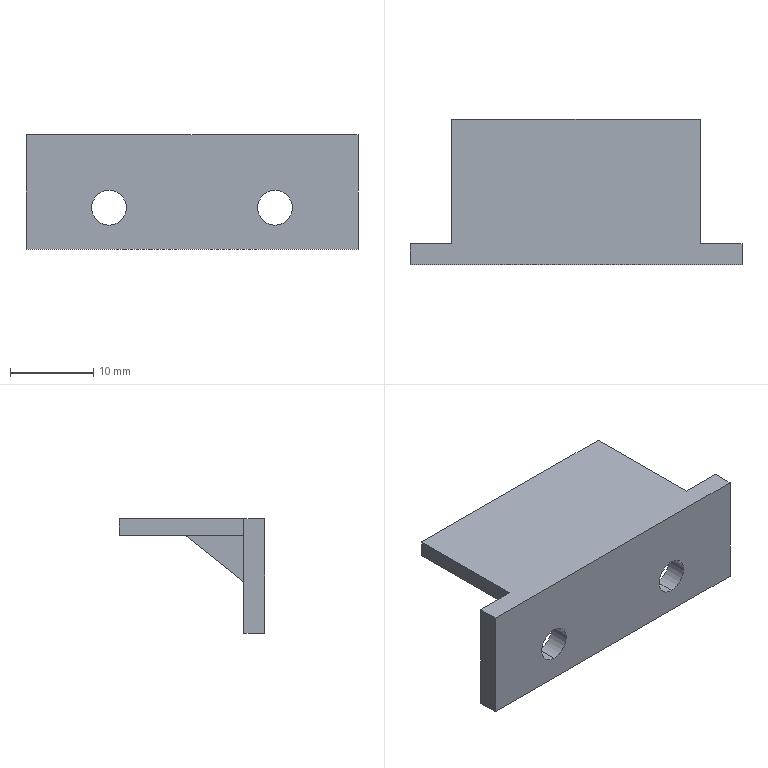Part | SolidWorks | features BaseBody 1 | 1 solid | 17 faces | box 40 x 17.5 x 13.8 mm | volume 2505 mm3 | plane 13 | cylinder 4 | commonest cylinder face diameters 4.2 x4
STEP:
#1=CARTESIAN_POINT('',(269.946,-4030.973,2013.371));
#2=VERTEX_POINT('',#1);
#3=CARTESIAN_POINT('',(269.946,-4030.973,2017.571));
#4=VERTEX_POINT('',#3);
#5=CARTESIAN_POINT('',(269.946,-4030.973,2015.471));
#6=DIRECTION('',(0.,1.,0.));
#7=DIRECTION('',(0.,0.,1.));
#8=AXIS2_PLACEMENT_3D('',#5,#6,#7);
#9=CIRCLE('',#8,2.1);
#10=EDGE_CURVE('',#2,#4,#9,.T.);
#11=ORIENTED_EDGE('',*,*,#10,.F.);
#12=CARTESIAN_POINT('',(269.946,-4028.473,2013.371));
#13=VERTEX_POINT('',#12);
#14=CARTESIAN_POINT('',(269.946,-4034.473,2013.371));
#15=DIRECTION('',(0.,1.,0.));
#16=VECTOR('',#15,1000.);
#17=LINE('',#14,#16);
#18=EDGE_CURVE('',#2,#13,#17,.T.);
#19=ORIENTED_EDGE('',*,*,#18,.T.);
#20=CARTESIAN_POINT('',(269.946,-4028.473,2017.571));
#21=VERTEX_POINT('',#20);
#22=CARTESIAN_POINT('',(269.946,-4028.473,2015.471));
#23=DIRECTION('',(0.,1.,0.));
#24=DIRECTION('',(0.,0.,1.));
#25=AXIS2_PLACEMENT_3D('',#22,#23,#24);
#26=CIRCLE('',#25,2.1);
#27=EDGE_CURVE('',#13,#21,#26,.T.);
#28=ORIENTED_EDGE('',*,*,#27,.T.);
#29=CARTESIAN_POINT('',(269.946,-4034.473,2017.571));
#30=DIRECTION('',(0.,1.,0.));
#31=VECTOR('',#30,1000.);
#32=LINE('',#29,#31);
#33=EDGE_CURVE('',#4,#21,#32,.T.);
#34=ORIENTED_EDGE('',*,*,#33,.F.);
#35=EDGE_LOOP('',(#11,#19,#28,#34));
#36=FACE_OUTER_BOUND('',#35,.T.);
#37=CARTESIAN_POINT('',(269.946,-4034.473,2015.471));
#38=DIRECTION('',(0.,1.,0.));
#39=DIRECTION('',(0.,0.,1.));
#40=AXIS2_PLACEMENT_3D('',#37,#38,#39);
#41=CYLINDRICAL_SURFACE('',#40,2.1);
#42=ADVANCED_FACE('',(#36),#41,.F.);
#43=CARTESIAN_POINT('',(249.946,-4030.973,2013.371));
#44=VERTEX_POINT('',#43);
#45=CARTESIAN_POINT('',(249.946,-4030.973,2017.571));
#46=VERTEX_POINT('',#45);
#47=CARTESIAN_POINT('',(249.946,-4030.973,2015.471));
#48=DIRECTION('',(0.,1.,0.));
#49=DIRECTION('',(0.,0.,1.));
#50=AXIS2_PLACEMENT_3D('',#47,#48,#49);
#51=CIRCLE('',#50,2.1);
#52=EDGE_CURVE('',#44,#46,#51,.T.);
#53=ORIENTED_EDGE('',*,*,#52,.F.);
#54=CARTESIAN_POINT('',(249.946,-4028.473,2013.371));
#55=VERTEX_POINT('',#54);
#56=CARTESIAN_POINT('',(249.946,-4034.473,2013.371));
#57=DIRECTION('',(0.,1.,0.));
#58=VECTOR('',#57,1000.);
#59=LINE('',#56,#58);
#60=EDGE_CURVE('',#44,#55,#59,.T.);
#61=ORIENTED_EDGE('',*,*,#60,.T.);
#62=CARTESIAN_POINT('',(249.946,-4028.473,2017.571));
#63=VERTEX_POINT('',#62);
#64=CARTESIAN_POINT('',(249.946,-4028.473,2015.471));
#65=DIRECTION('',(0.,1.,0.));
#66=DIRECTION('',(0.,0.,1.));
#67=AXIS2_PLACEMENT_3D('',#64,#65,#66);
#68=CIRCLE('',#67,2.1);
#69=EDGE_CURVE('',#55,#63,#68,.T.);
#70=ORIENTED_EDGE('',*,*,#69,.T.);
#71=CARTESIAN_POINT('',(249.946,-4034.473,2017.571));
#72=DIRECTION('',(0.,1.,0.));
#73=VECTOR('',#72,1000.);
#74=LINE('',#71,#73);
#75=EDGE_CURVE('',#46,#63,#74,.T.);
#76=ORIENTED_EDGE('',*,*,#75,.F.);
#77=EDGE_LOOP('',(#53,#61,#70,#76));
#78=FACE_OUTER_BOUND('',#77,.T.);
#79=CARTESIAN_POINT('',(249.946,-4034.473,2015.471));
#80=DIRECTION('',(0.,1.,0.));
#81=DIRECTION('',(0.,0.,1.));
#82=AXIS2_PLACEMENT_3D('',#79,#80,#81);
#83=CYLINDRICAL_SURFACE('',#82,2.1);
#84=ADVANCED_FACE('',(#78),#83,.F.);
#85=CARTESIAN_POINT('',(244.946,-4028.473,2024.271));
#86=VERTEX_POINT('',#85);
#87=CARTESIAN_POINT('',(239.946,-4028.473,2024.271));
#88=VERTEX_POINT('',#87);
#89=CARTESIAN_POINT('',(259.946,-4028.473,2024.271));
#90=DIRECTION('',(-1.,0.,0.));
#91=VECTOR('',#90,1000.);
#92=LINE('',#89,#91);
#93=EDGE_CURVE('',#86,#88,#92,.T.);
#94=ORIENTED_EDGE('',*,*,#93,.T.);
#95=CARTESIAN_POINT('',(239.946,-4030.973,2024.271));
#96=VERTEX_POINT('',#95);
#97=CARTESIAN_POINT('',(239.946,-4028.473,2024.271));
#98=DIRECTION('',(0.,-1.,0.));
#99=VECTOR('',#98,1000.);
#100=LINE('',#97,#99);
#101=EDGE_CURVE('',#88,#96,#100,.T.);
#102=ORIENTED_EDGE('',*,*,#101,.T.);
#103=CARTESIAN_POINT('',(279.946,-4030.973,2024.271));
#104=VERTEX_POINT('',#103);
#105=CARTESIAN_POINT('',(259.946,-4030.973,2024.271));
#106=DIRECTION('',(1.,0.,0.));
#107=VECTOR('',#106,1000.);
#108=LINE('',#105,#107);
#109=EDGE_CURVE('',#96,#104,#108,.T.);
#110=ORIENTED_EDGE('',*,*,#109,.T.);
#111=CARTESIAN_POINT('',(279.946,-4028.473,2024.271));
#112=VERTEX_POINT('',#111);
#113=CARTESIAN_POINT('',(279.946,-4028.473,2024.271));
#114=DIRECTION('',(0.,1.,0.));
#115=VECTOR('',#114,1000.);
#116=LINE('',#113,#115);
#117=EDGE_CURVE('',#104,#112,#116,.T.);
#118=ORIENTED_EDGE('',*,*,#117,.T.);
#119=CARTESIAN_POINT('',(274.946,-4028.473,2024.271));
#120=VERTEX_POINT('',#119);
#121=CARTESIAN_POINT('',(259.946,-4028.473,2024.271));
#122=DIRECTION('',(-1.,0.,0.));
#123=VECTOR('',#122,1000.);
#124=LINE('',#121,#123);
#125=EDGE_CURVE('',#112,#120,#124,.T.);
#126=ORIENTED_EDGE('',*,*,#125,.T.);
#127=CARTESIAN_POINT('',(274.946,-4013.473,2024.271));
#128=VERTEX_POINT('',#127);
#129=CARTESIAN_POINT('',(274.946,-4028.473,2024.271));
#130=DIRECTION('',(0.,1.,0.));
#131=VECTOR('',#130,1000.);
#132=LINE('',#129,#131);
#133=EDGE_CURVE('',#120,#128,#132,.T.);
#134=ORIENTED_EDGE('',*,*,#133,.T.);
#135=CARTESIAN_POINT('',(244.946,-4013.473,2024.271));
#136=VERTEX_POINT('',#135);
#137=CARTESIAN_POINT('',(259.946,-4013.473,2024.271));
#138=DIRECTION('',(-1.,0.,0.));
#139=VECTOR('',#138,1000.);
#140=LINE('',#137,#139);
#141=EDGE_CURVE('',#128,#136,#140,.T.);
#142=ORIENTED_EDGE('',*,*,#141,.T.);
#143=CARTESIAN_POINT('',(244.946,-4028.473,2024.271));
#144=DIRECTION('',(0.,-1.,0.));
#145=VECTOR('',#144,1000.);
#146=LINE('',#143,#145);
#147=EDGE_CURVE('',#136,#86,#146,.T.);
#148=ORIENTED_EDGE('',*,*,#147,.T.);
#149=EDGE_LOOP('',(#94,#102,#110,#118,#126,#134,#142,#148));
#150=FACE_OUTER_BOUND('',#149,.T.);
#151=CARTESIAN_POINT('',(259.946,-4028.473,2024.271));
#152=DIRECTION('',(0.,0.,1.));
#153=DIRECTION('',(0.,-1.,0.));
#154=AXIS2_PLACEMENT_3D('',#151,#152,#153);
#155=PLANE('',#154);
#156=ADVANCED_FACE('',(#150),#155,.T.);
#157=CARTESIAN_POINT('',(239.946,-4030.973,2010.471));
#158=VERTEX_POINT('',#157);
#159=CARTESIAN_POINT('',(239.946,-4030.973,2024.271));
#160=DIRECTION('',(0.,0.,1.));
#161=VECTOR('',#160,1000.);
#162=LINE('',#159,#161);
#163=EDGE_CURVE('',#158,#96,#162,.T.);
#164=ORIENTED_EDGE('',*,*,#163,.T.);
#165=ORIENTED_EDGE('',*,*,#101,.F.);
#166=CARTESIAN_POINT('',(239.946,-4028.473,2010.471));
#167=VERTEX_POINT('',#166);
#168=CARTESIAN_POINT('',(239.946,-4028.473,2024.271));
#169=DIRECTION('',(0.,0.,-1.));
#170=VECTOR('',#169,1000.);
#171=LINE('',#168,#170);
#172=EDGE_CURVE('',#88,#167,#171,.T.);
#173=ORIENTED_EDGE('',*,*,#172,.T.);
#174=CARTESIAN_POINT('',(239.946,-4034.473,2010.471));
#175=DIRECTION('',(0.,-1.,0.));
#176=VECTOR('',#175,1000.);
#177=LINE('',#174,#176);
#178=EDGE_CURVE('',#167,#158,#177,.T.);
#179=ORIENTED_EDGE('',*,*,#178,.T.);
#180=EDGE_LOOP('',(#164,#165,#173,#179));
#181=FACE_OUTER_BOUND('',#180,.T.);
#182=CARTESIAN_POINT('',(239.946,-4034.473,2024.271));
#183=DIRECTION('',(-1.,0.,0.));
#184=DIRECTION('',(0.,-1.,0.));
#185=AXIS2_PLACEMENT_3D('',#182,#183,#184);
#186=PLANE('',#185);
#187=ADVANCED_FACE('',(#181),#186,.T.);
#188=CARTESIAN_POINT('',(267.446,-4028.473,2016.671));
#189=VERTEX_POINT('',#188);
#190=CARTESIAN_POINT('',(252.446,-4028.473,2016.671));
#191=VERTEX_POINT('',#190);
#192=CARTESIAN_POINT('',(279.946,-4028.473,2016.671));
#193=DIRECTION('',(-1.,0.,0.));
#194=VECTOR('',#193,1000.);
#195=LINE('',#192,#194);
#196=EDGE_CURVE('',#189,#191,#195,.T.);
#197=ORIENTED_EDGE('',*,*,#196,.F.);
#198=CARTESIAN_POINT('',(267.446,-4028.473,2022.271));
#199=VERTEX_POINT('',#198);
#200=CARTESIAN_POINT('',(267.446,-4028.473,2024.271));
#201=DIRECTION('',(0.,0.,-1.));
#202=VECTOR('',#201,1000.);
#203=LINE('',#200,#202);
#204=EDGE_CURVE('',#199,#189,#203,.T.);
#205=ORIENTED_EDGE('',*,*,#204,.F.);
#206=CARTESIAN_POINT('',(274.946,-4028.473,2022.271));
#207=VERTEX_POINT('',#206);
#208=CARTESIAN_POINT('',(279.946,-4028.473,2022.271));
#209=DIRECTION('',(-1.,0.,0.));
#210=VECTOR('',#209,1000.);
#211=LINE('',#208,#210);
#212=EDGE_CURVE('',#207,#199,#211,.T.);
#213=ORIENTED_EDGE('',*,*,#212,.F.);
#214=CARTESIAN_POINT('',(274.946,-4028.473,2024.271));
#215=DIRECTION('',(0.,0.,-1.));
#216=VECTOR('',#215,1000.);
#217=LINE('',#214,#216);
#218=EDGE_CURVE('',#120,#207,#217,.T.);
#219=ORIENTED_EDGE('',*,*,#218,.F.);
#220=ORIENTED_EDGE('',*,*,#125,.F.);
#221=CARTESIAN_POINT('',(279.946,-4028.473,2010.471));
#222=VERTEX_POINT('',#221);
#223=CARTESIAN_POINT('',(279.946,-4028.473,2024.271));
#224=DIRECTION('',(0.,0.,1.));
#225=VECTOR('',#224,1000.);
#226=LINE('',#223,#225);
#227=EDGE_CURVE('',#222,#112,#226,.T.);
#228=ORIENTED_EDGE('',*,*,#227,.F.);
#229=CARTESIAN_POINT('',(279.946,-4028.473,2010.471));
#230=DIRECTION('',(1.,0.,0.));
#231=VECTOR('',#230,1000.);
#232=LINE('',#229,#231);
#233=EDGE_CURVE('',#167,#222,#232,.T.);
#234=ORIENTED_EDGE('',*,*,#233,.F.);
#235=ORIENTED_EDGE('',*,*,#172,.F.);
#236=ORIENTED_EDGE('',*,*,#93,.F.);
#237=CARTESIAN_POINT('',(244.946,-4028.473,2022.271));
#238=VERTEX_POINT('',#237);
#239=CARTESIAN_POINT('',(244.946,-4028.473,2024.271));
#240=DIRECTION('',(0.,0.,1.));
#241=VECTOR('',#240,1000.);
#242=LINE('',#239,#241);
#243=EDGE_CURVE('',#238,#86,#242,.T.);
#244=ORIENTED_EDGE('',*,*,#243,.F.);
#245=CARTESIAN_POINT('',(252.446,-4028.473,2022.271));
#246=VERTEX_POINT('',#245);
#247=CARTESIAN_POINT('',(279.946,-4028.473,2022.271));
#248=DIRECTION('',(-1.,0.,0.));
#249=VECTOR('',#248,1000.);
#250=LINE('',#247,#249);
#251=EDGE_CURVE('',#246,#238,#250,.T.);
#252=ORIENTED_EDGE('',*,*,#251,.F.);
#253=CARTESIAN_POINT('',(252.446,-4028.473,2024.271));
#254=DIRECTION('',(0.,0.,1.));
#255=VECTOR('',#254,1000.);
#256=LINE('',#253,#255);
#257=EDGE_CURVE('',#191,#246,#256,.T.);
#258=ORIENTED_EDGE('',*,*,#257,.F.);
#259=EDGE_LOOP('',(#197,#205,#213,#219,#220,#228,#234,#235,#236,#244,#252,#258));
#260=FACE_OUTER_BOUND('',#259,.T.);
#261=CARTESIAN_POINT('',(269.946,-4028.473,2015.471));
#262=DIRECTION('',(0.,1.,0.));
#263=DIRECTION('',(0.,0.,1.));
#264=AXIS2_PLACEMENT_3D('',#261,#262,#263);
#265=CIRCLE('',#264,2.1);
#266=EDGE_CURVE('',#21,#13,#265,.T.);
#267=ORIENTED_EDGE('',*,*,#266,.F.);
#268=ORIENTED_EDGE('',*,*,#27,.F.);
#269=EDGE_LOOP('',(#267,#268));
#270=FACE_BOUND('',#269,.T.);
#271=CARTESIAN_POINT('',(249.946,-4028.473,2015.471));
#272=DIRECTION('',(0.,1.,0.));
#273=DIRECTION('',(0.,0.,1.));
#274=AXIS2_PLACEMENT_3D('',#271,#272,#273);
#275=CIRCLE('',#274,2.1);
#276=EDGE_CURVE('',#63,#55,#275,.T.);
#277=ORIENTED_EDGE('',*,*,#276,.F.);
#278=ORIENTED_EDGE('',*,*,#69,.F.);
#279=EDGE_LOOP('',(#277,#278));
#280=FACE_BOUND('',#279,.T.);
#281=CARTESIAN_POINT('',(279.946,-4028.473,2024.271));
#282=DIRECTION('',(0.,-1.,0.));
#283=DIRECTION('',(0.,0.,-1.));
#284=AXIS2_PLACEMENT_3D('',#281,#282,#283);
#285=PLANE('',#284);
#286=ADVANCED_FACE('',(#260,#270,#280),#285,.F.);
#287=CARTESIAN_POINT('',(244.946,-4013.473,2022.271));
#288=VERTEX_POINT('',#287);
#289=CARTESIAN_POINT('',(244.946,-4013.473,2024.271));
#290=DIRECTION('',(0.,0.,-1.));
#291=VECTOR('',#290,1000.);
#292=LINE('',#289,#291);
#293=EDGE_CURVE('',#136,#288,#292,.T.);
#294=ORIENTED_EDGE('',*,*,#293,.T.);
#295=CARTESIAN_POINT('',(244.946,-4013.473,2022.271));
#296=DIRECTION('',(0.,-1.,0.));
#297=VECTOR('',#296,1000.);
#298=LINE('',#295,#297);
#299=EDGE_CURVE('',#288,#238,#298,.T.);
#300=ORIENTED_EDGE('',*,*,#299,.T.);
#301=ORIENTED_EDGE('',*,*,#243,.T.);
#302=ORIENTED_EDGE('',*,*,#147,.F.);
#303=EDGE_LOOP('',(#294,#300,#301,#302));
#304=FACE_OUTER_BOUND('',#303,.T.);
#305=CARTESIAN_POINT('',(244.946,-4013.473,2024.271));
#306=DIRECTION('',(-1.,0.,0.));
#307=DIRECTION('',(0.,-1.,0.));
#308=AXIS2_PLACEMENT_3D('',#305,#306,#307);
#309=PLANE('',#308);
#310=ADVANCED_FACE('',(#304),#309,.T.);
#311=ORIENTED_EDGE('',*,*,#141,.F.);
#312=CARTESIAN_POINT('',(274.946,-4013.473,2022.271));
#313=VERTEX_POINT('',#312);
#314=CARTESIAN_POINT('',(274.946,-4013.473,2024.271));
#315=DIRECTION('',(0.,0.,-1.));
#316=VECTOR('',#315,1000.);
#317=LINE('',#314,#316);
#318=EDGE_CURVE('',#128,#313,#317,.T.);
#319=ORIENTED_EDGE('',*,*,#318,.T.);
#320=CARTESIAN_POINT('',(274.946,-4013.473,2022.271));
#321=DIRECTION('',(-1.,0.,0.));
#322=VECTOR('',#321,1000.);
#323=LINE('',#320,#322);
#324=EDGE_CURVE('',#313,#288,#323,.T.);
#325=ORIENTED_EDGE('',*,*,#324,.T.);
#326=ORIENTED_EDGE('',*,*,#293,.F.);
#327=EDGE_LOOP('',(#311,#319,#325,#326));
#328=FACE_OUTER_BOUND('',#327,.T.);
#329=CARTESIAN_POINT('',(274.946,-4013.473,2024.271));
#330=DIRECTION('',(0.,1.,0.));
#331=DIRECTION('',(0.,0.,1.));
#332=AXIS2_PLACEMENT_3D('',#329,#330,#331);
#333=PLANE('',#332);
#334=ADVANCED_FACE('',(#328),#333,.T.);
#335=ORIENTED_EDGE('',*,*,#318,.F.);
#336=ORIENTED_EDGE('',*,*,#133,.F.);
#337=ORIENTED_EDGE('',*,*,#218,.T.);
#338=CARTESIAN_POINT('',(274.946,-4043.473,2022.271));
#339=DIRECTION('',(0.,1.,0.));
#340=VECTOR('',#339,1000.);
#341=LINE('',#338,#340);
#342=EDGE_CURVE('',#207,#313,#341,.T.);
#343=ORIENTED_EDGE('',*,*,#342,.T.);
#344=EDGE_LOOP('',(#335,#336,#337,#343));
#345=FACE_OUTER_BOUND('',#344,.T.);
#346=CARTESIAN_POINT('',(274.946,-4043.473,2024.271));
#347=DIRECTION('',(1.,0.,0.));
#348=DIRECTION('',(0.,1.,0.));
#349=AXIS2_PLACEMENT_3D('',#346,#347,#348);
#350=PLANE('',#349);
#351=ADVANCED_FACE('',(#345),#350,.T.);
#352=CARTESIAN_POINT('',(279.946,-4030.973,2010.471));
#353=VERTEX_POINT('',#352);
#354=CARTESIAN_POINT('',(279.946,-4030.973,2006.271));
#355=DIRECTION('',(0.,0.,-1.));
#356=VECTOR('',#355,1000.);
#357=LINE('',#354,#356);
#358=EDGE_CURVE('',#104,#353,#357,.T.);
#359=ORIENTED_EDGE('',*,*,#358,.T.);
#360=CARTESIAN_POINT('',(279.946,-4034.473,2010.471));
#361=DIRECTION('',(0.,1.,0.));
#362=VECTOR('',#361,1000.);
#363=LINE('',#360,#362);
#364=EDGE_CURVE('',#353,#222,#363,.T.);
#365=ORIENTED_EDGE('',*,*,#364,.T.);
#366=ORIENTED_EDGE('',*,*,#227,.T.);
#367=ORIENTED_EDGE('',*,*,#117,.F.);
#368=EDGE_LOOP('',(#359,#365,#366,#367));
#369=FACE_OUTER_BOUND('',#368,.T.);
#370=CARTESIAN_POINT('',(279.946,-4034.473,2006.271));
#371=DIRECTION('',(1.,0.,0.));
#372=DIRECTION('',(0.,1.,0.));
#373=AXIS2_PLACEMENT_3D('',#370,#371,#372);
#374=PLANE('',#373);
#375=ADVANCED_FACE('',(#369),#374,.T.);
#376=CARTESIAN_POINT('',(269.946,-4030.973,2015.471));
#377=DIRECTION('',(0.,1.,0.));
#378=DIRECTION('',(0.,0.,1.));
#379=AXIS2_PLACEMENT_3D('',#376,#377,#378);
#380=CIRCLE('',#379,2.1);
#381=EDGE_CURVE('',#4,#2,#380,.T.);
#382=ORIENTED_EDGE('',*,*,#381,.T.);
#383=ORIENTED_EDGE('',*,*,#10,.T.);
#384=EDGE_LOOP('',(#382,#383));
#385=FACE_BOUND('',#384,.T.);
#386=CARTESIAN_POINT('',(249.946,-4030.973,2015.471));
#387=DIRECTION('',(0.,1.,0.));
#388=DIRECTION('',(0.,0.,1.));
#389=AXIS2_PLACEMENT_3D('',#386,#387,#388);
#390=CIRCLE('',#389,2.1);
#391=EDGE_CURVE('',#46,#44,#390,.T.);
#392=ORIENTED_EDGE('',*,*,#391,.T.);
#393=ORIENTED_EDGE('',*,*,#52,.T.);
#394=EDGE_LOOP('',(#392,#393));
#395=FACE_BOUND('',#394,.T.);
#396=ORIENTED_EDGE('',*,*,#109,.F.);
#397=ORIENTED_EDGE('',*,*,#163,.F.);
#398=CARTESIAN_POINT('',(259.946,-4030.973,2010.471));
#399=DIRECTION('',(1.,0.,0.));
#400=VECTOR('',#399,1000.);
#401=LINE('',#398,#400);
#402=EDGE_CURVE('',#158,#353,#401,.T.);
#403=ORIENTED_EDGE('',*,*,#402,.T.);
#404=ORIENTED_EDGE('',*,*,#358,.F.);
#405=EDGE_LOOP('',(#396,#397,#403,#404));
#406=FACE_OUTER_BOUND('',#405,.T.);
#407=CARTESIAN_POINT('',(259.946,-4030.973,2015.271));
#408=DIRECTION('',(0.,-1.,0.));
#409=DIRECTION('',(0.,0.,-1.));
#410=AXIS2_PLACEMENT_3D('',#407,#408,#409);
#411=PLANE('',#410);
#412=ADVANCED_FACE('',(#385,#395,#406),#411,.T.);
#413=ORIENTED_EDGE('',*,*,#402,.F.);
#414=ORIENTED_EDGE('',*,*,#178,.F.);
#415=ORIENTED_EDGE('',*,*,#233,.T.);
#416=ORIENTED_EDGE('',*,*,#364,.F.);
#417=EDGE_LOOP('',(#413,#414,#415,#416));
#418=FACE_OUTER_BOUND('',#417,.T.);
#419=CARTESIAN_POINT('',(239.946,-4030.973,2010.471));
#420=DIRECTION('',(0.,0.,-1.));
#421=DIRECTION('',(0.,1.,0.));
#422=AXIS2_PLACEMENT_3D('',#419,#420,#421);
#423=PLANE('',#422);
#424=ADVANCED_FACE('',(#418),#423,.T.);
#425=CARTESIAN_POINT('',(252.446,-4021.473,2022.271));
#426=VERTEX_POINT('',#425);
#427=CARTESIAN_POINT('',(252.446,-4021.473,2022.271));
#428=DIRECTION('',(0.,-0.7809,-0.6247));
#429=VECTOR('',#428,1000.);
#430=LINE('',#427,#429);
#431=EDGE_CURVE('',#426,#191,#430,.T.);
#432=ORIENTED_EDGE('',*,*,#431,.T.);
#433=ORIENTED_EDGE('',*,*,#257,.T.);
#434=CARTESIAN_POINT('',(252.446,-4021.473,2022.271));
#435=DIRECTION('',(0.,1.,0.));
#436=VECTOR('',#435,1000.);
#437=LINE('',#434,#436);
#438=EDGE_CURVE('',#246,#426,#437,.T.);
#439=ORIENTED_EDGE('',*,*,#438,.T.);
#440=EDGE_LOOP('',(#432,#433,#439));
#441=FACE_OUTER_BOUND('',#440,.T.);
#442=CARTESIAN_POINT('',(252.446,-4021.473,2022.271));
#443=DIRECTION('',(-1.,0.,0.));
#444=DIRECTION('',(0.,-1.,0.));
#445=AXIS2_PLACEMENT_3D('',#442,#443,#444);
#446=PLANE('',#445);
#447=ADVANCED_FACE('',(#441),#446,.T.);
#448=CARTESIAN_POINT('',(267.446,-4021.473,2022.271));
#449=VERTEX_POINT('',#448);
#450=CARTESIAN_POINT('',(267.446,-4031.473,2014.271));
#451=DIRECTION('',(0.,-0.7809,-0.6247));
#452=VECTOR('',#451,1000.);
#453=LINE('',#450,#452);
#454=EDGE_CURVE('',#449,#189,#453,.T.);
#455=ORIENTED_EDGE('',*,*,#454,.T.);
#456=ORIENTED_EDGE('',*,*,#196,.T.);
#457=ORIENTED_EDGE('',*,*,#431,.F.);
#458=CARTESIAN_POINT('',(267.446,-4021.473,2022.271));
#459=DIRECTION('',(1.,0.,0.));
#460=VECTOR('',#459,1000.);
#461=LINE('',#458,#460);
#462=EDGE_CURVE('',#426,#449,#461,.T.);
#463=ORIENTED_EDGE('',*,*,#462,.T.);
#464=EDGE_LOOP('',(#455,#456,#457,#463));
#465=FACE_OUTER_BOUND('',#464,.T.);
#466=CARTESIAN_POINT('',(267.446,-4031.473,2014.271));
#467=DIRECTION('',(0.,0.6247,-0.7809));
#468=DIRECTION('',(0.,0.7809,0.6247));
#469=AXIS2_PLACEMENT_3D('',#466,#467,#468);
#470=PLANE('',#469);
#471=ADVANCED_FACE('',(#465),#470,.T.);
#472=CARTESIAN_POINT('',(267.446,-4028.14,2022.271));
#473=DIRECTION('',(0.,1.,0.));
#474=VECTOR('',#473,1000.);
#475=LINE('',#472,#474);
#476=EDGE_CURVE('',#199,#449,#475,.T.);
#477=ORIENTED_EDGE('',*,*,#476,.F.);
#478=ORIENTED_EDGE('',*,*,#204,.T.);
#479=ORIENTED_EDGE('',*,*,#454,.F.);
#480=EDGE_LOOP('',(#477,#478,#479));
#481=FACE_OUTER_BOUND('',#480,.T.);
#482=CARTESIAN_POINT('',(267.446,-4028.14,2019.605));
#483=DIRECTION('',(-1.,0.,0.));
#484=DIRECTION('',(0.,-1.,0.));
#485=AXIS2_PLACEMENT_3D('',#482,#483,#484);
#486=PLANE('',#485);
#487=ADVANCED_FACE('',(#481),#486,.F.);
#488=ORIENTED_EDGE('',*,*,#251,.T.);
#489=ORIENTED_EDGE('',*,*,#299,.F.);
#490=ORIENTED_EDGE('',*,*,#324,.F.);
#491=ORIENTED_EDGE('',*,*,#342,.F.);
#492=ORIENTED_EDGE('',*,*,#212,.T.);
#493=ORIENTED_EDGE('',*,*,#476,.T.);
#494=ORIENTED_EDGE('',*,*,#462,.F.);
#495=ORIENTED_EDGE('',*,*,#438,.F.);
#496=EDGE_LOOP('',(#488,#489,#490,#491,#492,#493,#494,#495));
#497=FACE_OUTER_BOUND('',#496,.T.);
#498=CARTESIAN_POINT('',(244.946,-4013.473,2022.271));
#499=DIRECTION('',(0.,0.,1.));
#500=DIRECTION('',(0.,-1.,0.));
#501=AXIS2_PLACEMENT_3D('',#498,#499,#500);
#502=PLANE('',#501);
#503=ADVANCED_FACE('',(#497),#502,.F.);
#504=ORIENTED_EDGE('',*,*,#18,.F.);
#505=ORIENTED_EDGE('',*,*,#381,.F.);
#506=ORIENTED_EDGE('',*,*,#33,.T.);
#507=ORIENTED_EDGE('',*,*,#266,.T.);
#508=EDGE_LOOP('',(#504,#505,#506,#507));
#509=FACE_OUTER_BOUND('',#508,.T.);
#510=CARTESIAN_POINT('',(269.946,-4034.473,2015.471));
#511=DIRECTION('',(0.,1.,0.));
#512=DIRECTION('',(0.,0.,1.));
#513=AXIS2_PLACEMENT_3D('',#510,#511,#512);
#514=CYLINDRICAL_SURFACE('',#513,2.1);
#515=ADVANCED_FACE('',(#509),#514,.F.);
#516=ORIENTED_EDGE('',*,*,#60,.F.);
#517=ORIENTED_EDGE('',*,*,#391,.F.);
#518=ORIENTED_EDGE('',*,*,#75,.T.);
#519=ORIENTED_EDGE('',*,*,#276,.T.);
#520=EDGE_LOOP('',(#516,#517,#518,#519));
#521=FACE_OUTER_BOUND('',#520,.T.);
#522=CARTESIAN_POINT('',(249.946,-4034.473,2015.471));
#523=DIRECTION('',(0.,1.,0.));
#524=DIRECTION('',(0.,0.,1.));
#525=AXIS2_PLACEMENT_3D('',#522,#523,#524);
#526=CYLINDRICAL_SURFACE('',#525,2.1);
#527=ADVANCED_FACE('',(#521),#526,.F.);
#528=CLOSED_SHELL('',(#42,#84,#156,#187,#286,#310,#334,#351,#375,#412,#424,#447,#471,#487,#503,#515,#527));
#529=MANIFOLD_SOLID_BREP('',#528);
#530=CARTESIAN_POINT('',(0.,0.,0.));
#531=DIRECTION('',(0.,0.,1.));
#532=DIRECTION('',(1.,0.,0.));
#533=AXIS2_PLACEMENT_3D('',#530,#531,#532);
#534=(LENGTH_UNIT()NAMED_UNIT(*)SI_UNIT(.MILLI.,.METRE.));
#535=UNCERTAINTY_MEASURE_WITH_UNIT(LENGTH_MEASURE(0.00001),#534,'','');
#536=(NAMED_UNIT(*)PLANE_ANGLE_UNIT()SI_UNIT($,.RADIAN.));
#537=(NAMED_UNIT(*)SI_UNIT($,.STERADIAN.)SOLID_ANGLE_UNIT());
#538=(GEOMETRIC_REPRESENTATION_CONTEXT(3)GLOBAL_UNCERTAINTY_ASSIGNED_CONTEXT((#535))GLOBAL_UNIT_ASSIGNED_CONTEXT((#534,#536,#537))REPRESENTATION_CONTEXT('',''));
#539=ADVANCED_BREP_SHAPE_REPRESENTATION('',(#529,#533),#538);